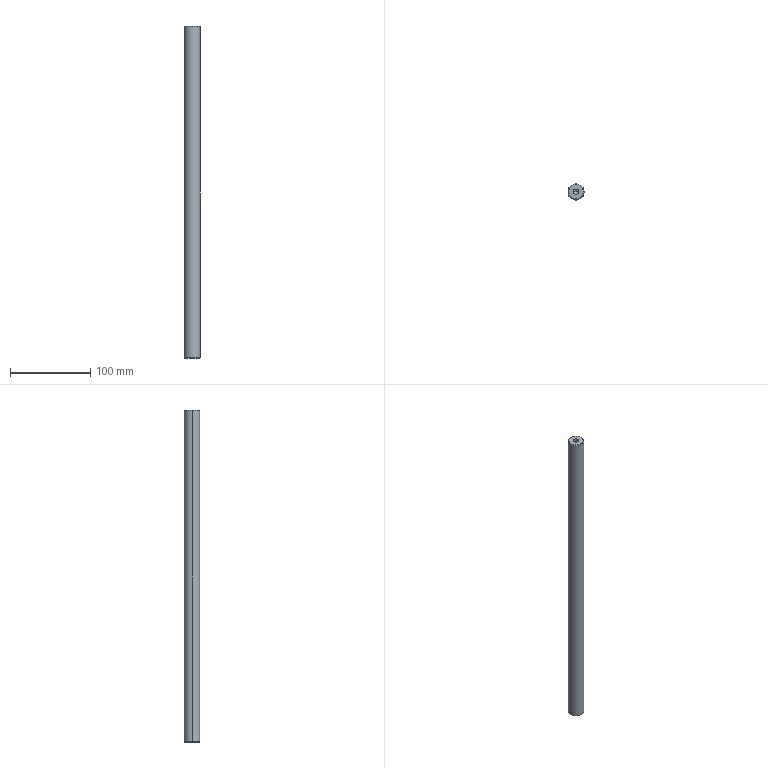Part | SolidWorks | features HoleWzd 2, Chamfer 1, Extrusion 1 | 1 solid | 16 faces | box 20 x 20 x 415 mm | volume 128650 mm3 | cone 8 | cylinder 6 | plane 2 | commonest cylinder face diameters 6.8 x4 20 x2
STEP:
#1=CARTESIAN_POINT('',(3.4,0.,22.25));
#2=VERTEX_POINT('',#1);
#3=CARTESIAN_POINT('',(-3.4,0.,22.25));
#4=VERTEX_POINT('',#3);
#5=CARTESIAN_POINT('',(0.,0.,22.25));
#6=DIRECTION('',(0.,0.,-1.));
#7=DIRECTION('',(-1.,0.,0.));
#8=AXIS2_PLACEMENT_3D('',#5,#6,#7);
#9=CIRCLE('',#8,3.4);
#10=EDGE_CURVE('',#2,#4,#9,.T.);
#11=ORIENTED_EDGE('',*,*,#10,.F.);
#12=CARTESIAN_POINT('',(3.4,0.,0.));
#13=VERTEX_POINT('',#12);
#14=CARTESIAN_POINT('',(3.4,0.,0.));
#15=DIRECTION('',(0.,0.,-1.));
#16=VECTOR('',#15,1000.);
#17=LINE('',#14,#16);
#18=EDGE_CURVE('',#2,#13,#17,.T.);
#19=ORIENTED_EDGE('',*,*,#18,.T.);
#20=CARTESIAN_POINT('',(-3.4,0.,0.));
#21=VERTEX_POINT('',#20);
#22=CARTESIAN_POINT('',(0.,0.,0.));
#23=DIRECTION('',(0.,0.,-1.));
#24=DIRECTION('',(-1.,0.,0.));
#25=AXIS2_PLACEMENT_3D('',#22,#23,#24);
#26=CIRCLE('',#25,3.4);
#27=EDGE_CURVE('',#13,#21,#26,.T.);
#28=ORIENTED_EDGE('',*,*,#27,.T.);
#29=CARTESIAN_POINT('',(-3.4,0.,0.));
#30=DIRECTION('',(0.,0.,-1.));
#31=VECTOR('',#30,1000.);
#32=LINE('',#29,#31);
#33=EDGE_CURVE('',#4,#21,#32,.T.);
#34=ORIENTED_EDGE('',*,*,#33,.F.);
#35=EDGE_LOOP('',(#11,#19,#28,#34));
#36=FACE_OUTER_BOUND('',#35,.T.);
#37=CARTESIAN_POINT('',(0.,0.,0.));
#38=DIRECTION('',(0.,0.,-1.));
#39=DIRECTION('',(-1.,0.,0.));
#40=AXIS2_PLACEMENT_3D('',#37,#38,#39);
#41=CYLINDRICAL_SURFACE('',#40,3.4);
#42=ADVANCED_FACE('',(#36),#41,.F.);
#43=CARTESIAN_POINT('',(0.,0.,24.293));
#44=VERTEX_POINT('',#43);
#45=CARTESIAN_POINT('',(-3.4,0.,22.25));
#46=DIRECTION('',(-0.8572,0.,-0.515));
#47=VECTOR('',#46,1000.);
#48=LINE('',#45,#47);
#49=EDGE_CURVE('',#44,#4,#48,.T.);
#50=ORIENTED_EDGE('',*,*,#49,.F.);
#51=CARTESIAN_POINT('',(3.4,0.,22.25));
#52=DIRECTION('',(0.8572,0.,-0.515));
#53=VECTOR('',#52,1000.);
#54=LINE('',#51,#53);
#55=EDGE_CURVE('',#44,#2,#54,.T.);
#56=ORIENTED_EDGE('',*,*,#55,.T.);
#57=ORIENTED_EDGE('',*,*,#10,.T.);
#58=EDGE_LOOP('',(#50,#56,#57));
#59=FACE_OUTER_BOUND('',#58,.T.);
#60=CARTESIAN_POINT('',(0.,0.,22.25));
#61=DIRECTION('',(0.,0.,-1.));
#62=DIRECTION('',(-1.,0.,0.));
#63=AXIS2_PLACEMENT_3D('',#60,#61,#62);
#64=CONICAL_SURFACE('',#63,3.4,1.03);
#65=ADVANCED_FACE('',(#59),#64,.F.);
#66=CARTESIAN_POINT('',(9.,0.,415.));
#67=VERTEX_POINT('',#66);
#68=CARTESIAN_POINT('',(-9.,0.,415.));
#69=VERTEX_POINT('',#68);
#70=CARTESIAN_POINT('',(0.,0.,415.));
#71=DIRECTION('',(0.,0.,1.));
#72=DIRECTION('',(1.,0.,0.));
#73=AXIS2_PLACEMENT_3D('',#70,#71,#72);
#74=CIRCLE('',#73,9.);
#75=EDGE_CURVE('',#67,#69,#74,.T.);
#76=ORIENTED_EDGE('',*,*,#75,.F.);
#77=CARTESIAN_POINT('',(10.,0.,414.));
#78=VERTEX_POINT('',#77);
#79=CARTESIAN_POINT('',(9.,0.,415.));
#80=DIRECTION('',(0.7071,0.,-0.7071));
#81=VECTOR('',#80,1000.);
#82=LINE('',#79,#81);
#83=EDGE_CURVE('',#67,#78,#82,.T.);
#84=ORIENTED_EDGE('',*,*,#83,.T.);
#85=CARTESIAN_POINT('',(-10.,0.,414.));
#86=VERTEX_POINT('',#85);
#87=CARTESIAN_POINT('',(0.,0.,414.));
#88=DIRECTION('',(0.,0.,-1.));
#89=DIRECTION('',(1.,0.,0.));
#90=AXIS2_PLACEMENT_3D('',#87,#88,#89);
#91=CIRCLE('',#90,10.);
#92=EDGE_CURVE('',#86,#78,#91,.T.);
#93=ORIENTED_EDGE('',*,*,#92,.F.);
#94=CARTESIAN_POINT('',(-9.,0.,415.));
#95=DIRECTION('',(-0.7071,0.,-0.7071));
#96=VECTOR('',#95,1000.);
#97=LINE('',#94,#96);
#98=EDGE_CURVE('',#69,#86,#97,.T.);
#99=ORIENTED_EDGE('',*,*,#98,.F.);
#100=EDGE_LOOP('',(#76,#84,#93,#99));
#101=FACE_OUTER_BOUND('',#100,.T.);
#102=CARTESIAN_POINT('',(0.,0.,415.));
#103=DIRECTION('',(0.,0.,-1.));
#104=DIRECTION('',(-1.,0.,0.));
#105=AXIS2_PLACEMENT_3D('',#102,#103,#104);
#106=CONICAL_SURFACE('',#105,9.,0.7854);
#107=ADVANCED_FACE('',(#101),#106,.T.);
#108=CARTESIAN_POINT('',(-9.,0.,0.));
#109=VERTEX_POINT('',#108);
#110=CARTESIAN_POINT('',(9.,0.,0.));
#111=VERTEX_POINT('',#110);
#112=CARTESIAN_POINT('',(0.,0.,0.));
#113=DIRECTION('',(0.,0.,-1.));
#114=DIRECTION('',(1.,0.,0.));
#115=AXIS2_PLACEMENT_3D('',#112,#113,#114);
#116=CIRCLE('',#115,9.);
#117=EDGE_CURVE('',#109,#111,#116,.T.);
#118=ORIENTED_EDGE('',*,*,#117,.F.);
#119=CARTESIAN_POINT('',(-10.,0.,1.));
#120=VERTEX_POINT('',#119);
#121=CARTESIAN_POINT('',(-10.,0.,1.));
#122=DIRECTION('',(-0.7071,0.,0.7071));
#123=VECTOR('',#122,1000.);
#124=LINE('',#121,#123);
#125=EDGE_CURVE('',#109,#120,#124,.T.);
#126=ORIENTED_EDGE('',*,*,#125,.T.);
#127=CARTESIAN_POINT('',(10.,0.,1.));
#128=VERTEX_POINT('',#127);
#129=CARTESIAN_POINT('',(0.,0.,1.));
#130=DIRECTION('',(0.,0.,1.));
#131=DIRECTION('',(1.,0.,0.));
#132=AXIS2_PLACEMENT_3D('',#129,#130,#131);
#133=CIRCLE('',#132,10.);
#134=EDGE_CURVE('',#128,#120,#133,.T.);
#135=ORIENTED_EDGE('',*,*,#134,.F.);
#136=CARTESIAN_POINT('',(10.,0.,1.));
#137=DIRECTION('',(0.7071,0.,0.7071));
#138=VECTOR('',#137,1000.);
#139=LINE('',#136,#138);
#140=EDGE_CURVE('',#111,#128,#139,.T.);
#141=ORIENTED_EDGE('',*,*,#140,.F.);
#142=EDGE_LOOP('',(#118,#126,#135,#141));
#143=FACE_OUTER_BOUND('',#142,.T.);
#144=CARTESIAN_POINT('',(0.,0.,1.));
#145=DIRECTION('',(0.,0.,1.));
#146=DIRECTION('',(1.,0.,0.));
#147=AXIS2_PLACEMENT_3D('',#144,#145,#146);
#148=CONICAL_SURFACE('',#147,10.,0.7854);
#149=ADVANCED_FACE('',(#143),#148,.T.);
#150=CARTESIAN_POINT('',(-3.4,0.,392.75));
#151=VERTEX_POINT('',#150);
#152=CARTESIAN_POINT('',(3.4,0.,392.75));
#153=VERTEX_POINT('',#152);
#154=CARTESIAN_POINT('',(0.,0.,392.75));
#155=DIRECTION('',(0.,0.,1.));
#156=DIRECTION('',(1.,0.,0.));
#157=AXIS2_PLACEMENT_3D('',#154,#155,#156);
#158=CIRCLE('',#157,3.4);
#159=EDGE_CURVE('',#151,#153,#158,.T.);
#160=ORIENTED_EDGE('',*,*,#159,.F.);
#161=CARTESIAN_POINT('',(-3.4,0.,415.));
#162=VERTEX_POINT('',#161);
#163=CARTESIAN_POINT('',(-3.4,0.,415.));
#164=DIRECTION('',(0.,0.,1.));
#165=VECTOR('',#164,1000.);
#166=LINE('',#163,#165);
#167=EDGE_CURVE('',#151,#162,#166,.T.);
#168=ORIENTED_EDGE('',*,*,#167,.T.);
#169=CARTESIAN_POINT('',(3.4,0.,415.));
#170=VERTEX_POINT('',#169);
#171=CARTESIAN_POINT('',(0.,0.,415.));
#172=DIRECTION('',(0.,0.,1.));
#173=DIRECTION('',(1.,0.,0.));
#174=AXIS2_PLACEMENT_3D('',#171,#172,#173);
#175=CIRCLE('',#174,3.4);
#176=EDGE_CURVE('',#162,#170,#175,.T.);
#177=ORIENTED_EDGE('',*,*,#176,.T.);
#178=CARTESIAN_POINT('',(3.4,0.,415.));
#179=DIRECTION('',(0.,0.,1.));
#180=VECTOR('',#179,1000.);
#181=LINE('',#178,#180);
#182=EDGE_CURVE('',#153,#170,#181,.T.);
#183=ORIENTED_EDGE('',*,*,#182,.F.);
#184=EDGE_LOOP('',(#160,#168,#177,#183));
#185=FACE_OUTER_BOUND('',#184,.T.);
#186=CARTESIAN_POINT('',(0.,0.,415.));
#187=DIRECTION('',(0.,0.,1.));
#188=DIRECTION('',(1.,0.,0.));
#189=AXIS2_PLACEMENT_3D('',#186,#187,#188);
#190=CYLINDRICAL_SURFACE('',#189,3.4);
#191=ADVANCED_FACE('',(#185),#190,.F.);
#192=CARTESIAN_POINT('',(0.,0.,390.707));
#193=VERTEX_POINT('',#192);
#194=CARTESIAN_POINT('',(3.4,0.,392.75));
#195=DIRECTION('',(0.8572,0.,0.515));
#196=VECTOR('',#195,1000.);
#197=LINE('',#194,#196);
#198=EDGE_CURVE('',#193,#153,#197,.T.);
#199=ORIENTED_EDGE('',*,*,#198,.F.);
#200=CARTESIAN_POINT('',(-3.4,0.,392.75));
#201=DIRECTION('',(-0.8572,0.,0.515));
#202=VECTOR('',#201,1000.);
#203=LINE('',#200,#202);
#204=EDGE_CURVE('',#193,#151,#203,.T.);
#205=ORIENTED_EDGE('',*,*,#204,.T.);
#206=ORIENTED_EDGE('',*,*,#159,.T.);
#207=EDGE_LOOP('',(#199,#205,#206));
#208=FACE_OUTER_BOUND('',#207,.T.);
#209=CARTESIAN_POINT('',(0.,0.,392.75));
#210=DIRECTION('',(0.,0.,1.));
#211=DIRECTION('',(1.,0.,0.));
#212=AXIS2_PLACEMENT_3D('',#209,#210,#211);
#213=CONICAL_SURFACE('',#212,3.4,1.03);
#214=ADVANCED_FACE('',(#208),#213,.F.);
#215=ORIENTED_EDGE('',*,*,#92,.T.);
#216=CARTESIAN_POINT('',(10.,0.,415.));
#217=DIRECTION('',(0.,0.,-1.));
#218=VECTOR('',#217,1000.);
#219=LINE('',#216,#218);
#220=EDGE_CURVE('',#78,#128,#219,.T.);
#221=ORIENTED_EDGE('',*,*,#220,.T.);
#222=ORIENTED_EDGE('',*,*,#134,.T.);
#223=CARTESIAN_POINT('',(-10.,0.,415.));
#224=DIRECTION('',(0.,0.,-1.));
#225=VECTOR('',#224,1000.);
#226=LINE('',#223,#225);
#227=EDGE_CURVE('',#86,#120,#226,.T.);
#228=ORIENTED_EDGE('',*,*,#227,.F.);
#229=EDGE_LOOP('',(#215,#221,#222,#228));
#230=FACE_OUTER_BOUND('',#229,.T.);
#231=CARTESIAN_POINT('',(0.,0.,415.));
#232=DIRECTION('',(0.,0.,-1.));
#233=DIRECTION('',(-1.,0.,0.));
#234=AXIS2_PLACEMENT_3D('',#231,#232,#233);
#235=CYLINDRICAL_SURFACE('',#234,10.);
#236=ADVANCED_FACE('',(#230),#235,.T.);
#237=ORIENTED_EDGE('',*,*,#220,.F.);
#238=CARTESIAN_POINT('',(0.,0.,414.));
#239=DIRECTION('',(0.,0.,-1.));
#240=DIRECTION('',(1.,0.,0.));
#241=AXIS2_PLACEMENT_3D('',#238,#239,#240);
#242=CIRCLE('',#241,10.);
#243=EDGE_CURVE('',#78,#86,#242,.T.);
#244=ORIENTED_EDGE('',*,*,#243,.T.);
#245=ORIENTED_EDGE('',*,*,#227,.T.);
#246=CARTESIAN_POINT('',(0.,0.,1.));
#247=DIRECTION('',(0.,0.,1.));
#248=DIRECTION('',(1.,0.,0.));
#249=AXIS2_PLACEMENT_3D('',#246,#247,#248);
#250=CIRCLE('',#249,10.);
#251=EDGE_CURVE('',#120,#128,#250,.T.);
#252=ORIENTED_EDGE('',*,*,#251,.T.);
#253=EDGE_LOOP('',(#237,#244,#245,#252));
#254=FACE_OUTER_BOUND('',#253,.T.);
#255=CARTESIAN_POINT('',(0.,0.,415.));
#256=DIRECTION('',(0.,0.,-1.));
#257=DIRECTION('',(-1.,0.,0.));
#258=AXIS2_PLACEMENT_3D('',#255,#256,#257);
#259=CYLINDRICAL_SURFACE('',#258,10.);
#260=ADVANCED_FACE('',(#254),#259,.T.);
#261=CARTESIAN_POINT('',(0.,0.,415.));
#262=DIRECTION('',(0.,0.,1.));
#263=DIRECTION('',(1.,0.,0.));
#264=AXIS2_PLACEMENT_3D('',#261,#262,#263);
#265=CIRCLE('',#264,9.);
#266=EDGE_CURVE('',#69,#67,#265,.T.);
#267=ORIENTED_EDGE('',*,*,#266,.T.);
#268=ORIENTED_EDGE('',*,*,#75,.T.);
#269=EDGE_LOOP('',(#267,#268));
#270=FACE_OUTER_BOUND('',#269,.T.);
#271=CARTESIAN_POINT('',(0.,0.,415.));
#272=DIRECTION('',(0.,0.,1.));
#273=DIRECTION('',(1.,0.,0.));
#274=AXIS2_PLACEMENT_3D('',#271,#272,#273);
#275=CIRCLE('',#274,3.4);
#276=EDGE_CURVE('',#170,#162,#275,.T.);
#277=ORIENTED_EDGE('',*,*,#276,.F.);
#278=ORIENTED_EDGE('',*,*,#176,.F.);
#279=EDGE_LOOP('',(#277,#278));
#280=FACE_BOUND('',#279,.T.);
#281=CARTESIAN_POINT('',(0.,0.,415.));
#282=DIRECTION('',(0.,0.,1.));
#283=DIRECTION('',(1.,0.,0.));
#284=AXIS2_PLACEMENT_3D('',#281,#282,#283);
#285=PLANE('',#284);
#286=ADVANCED_FACE('',(#270,#280),#285,.T.);
#287=CARTESIAN_POINT('',(0.,0.,0.));
#288=DIRECTION('',(0.,0.,-1.));
#289=DIRECTION('',(-1.,0.,0.));
#290=AXIS2_PLACEMENT_3D('',#287,#288,#289);
#291=CIRCLE('',#290,3.4);
#292=EDGE_CURVE('',#21,#13,#291,.T.);
#293=ORIENTED_EDGE('',*,*,#292,.F.);
#294=ORIENTED_EDGE('',*,*,#27,.F.);
#295=EDGE_LOOP('',(#293,#294));
#296=FACE_BOUND('',#295,.T.);
#297=CARTESIAN_POINT('',(0.,0.,0.));
#298=DIRECTION('',(0.,0.,-1.));
#299=DIRECTION('',(1.,0.,0.));
#300=AXIS2_PLACEMENT_3D('',#297,#298,#299);
#301=CIRCLE('',#300,9.);
#302=EDGE_CURVE('',#111,#109,#301,.T.);
#303=ORIENTED_EDGE('',*,*,#302,.T.);
#304=ORIENTED_EDGE('',*,*,#117,.T.);
#305=EDGE_LOOP('',(#303,#304));
#306=FACE_OUTER_BOUND('',#305,.T.);
#307=CARTESIAN_POINT('',(0.,0.,0.));
#308=DIRECTION('',(0.,0.,1.));
#309=DIRECTION('',(1.,0.,0.));
#310=AXIS2_PLACEMENT_3D('',#307,#308,#309);
#311=PLANE('',#310);
#312=ADVANCED_FACE('',(#296,#306),#311,.F.);
#313=ORIENTED_EDGE('',*,*,#204,.F.);
#314=ORIENTED_EDGE('',*,*,#198,.T.);
#315=CARTESIAN_POINT('',(0.,0.,392.75));
#316=DIRECTION('',(0.,0.,1.));
#317=DIRECTION('',(1.,0.,0.));
#318=AXIS2_PLACEMENT_3D('',#315,#316,#317);
#319=CIRCLE('',#318,3.4);
#320=EDGE_CURVE('',#153,#151,#319,.T.);
#321=ORIENTED_EDGE('',*,*,#320,.T.);
#322=EDGE_LOOP('',(#313,#314,#321));
#323=FACE_OUTER_BOUND('',#322,.T.);
#324=CARTESIAN_POINT('',(0.,0.,392.75));
#325=DIRECTION('',(0.,0.,1.));
#326=DIRECTION('',(1.,0.,0.));
#327=AXIS2_PLACEMENT_3D('',#324,#325,#326);
#328=CONICAL_SURFACE('',#327,3.4,1.03);
#329=ADVANCED_FACE('',(#323),#328,.F.);
#330=ORIENTED_EDGE('',*,*,#167,.F.);
#331=ORIENTED_EDGE('',*,*,#320,.F.);
#332=ORIENTED_EDGE('',*,*,#182,.T.);
#333=ORIENTED_EDGE('',*,*,#276,.T.);
#334=EDGE_LOOP('',(#330,#331,#332,#333));
#335=FACE_OUTER_BOUND('',#334,.T.);
#336=CARTESIAN_POINT('',(0.,0.,415.));
#337=DIRECTION('',(0.,0.,1.));
#338=DIRECTION('',(1.,0.,0.));
#339=AXIS2_PLACEMENT_3D('',#336,#337,#338);
#340=CYLINDRICAL_SURFACE('',#339,3.4);
#341=ADVANCED_FACE('',(#335),#340,.F.);
#342=ORIENTED_EDGE('',*,*,#125,.F.);
#343=ORIENTED_EDGE('',*,*,#302,.F.);
#344=ORIENTED_EDGE('',*,*,#140,.T.);
#345=ORIENTED_EDGE('',*,*,#251,.F.);
#346=EDGE_LOOP('',(#342,#343,#344,#345));
#347=FACE_OUTER_BOUND('',#346,.T.);
#348=CARTESIAN_POINT('',(0.,0.,1.));
#349=DIRECTION('',(0.,0.,1.));
#350=DIRECTION('',(1.,0.,0.));
#351=AXIS2_PLACEMENT_3D('',#348,#349,#350);
#352=CONICAL_SURFACE('',#351,10.,0.7854);
#353=ADVANCED_FACE('',(#347),#352,.T.);
#354=ORIENTED_EDGE('',*,*,#83,.F.);
#355=ORIENTED_EDGE('',*,*,#266,.F.);
#356=ORIENTED_EDGE('',*,*,#98,.T.);
#357=ORIENTED_EDGE('',*,*,#243,.F.);
#358=EDGE_LOOP('',(#354,#355,#356,#357));
#359=FACE_OUTER_BOUND('',#358,.T.);
#360=CARTESIAN_POINT('',(0.,0.,415.));
#361=DIRECTION('',(0.,0.,-1.));
#362=DIRECTION('',(-1.,0.,0.));
#363=AXIS2_PLACEMENT_3D('',#360,#361,#362);
#364=CONICAL_SURFACE('',#363,9.,0.7854);
#365=ADVANCED_FACE('',(#359),#364,.T.);
#366=ORIENTED_EDGE('',*,*,#55,.F.);
#367=ORIENTED_EDGE('',*,*,#49,.T.);
#368=CARTESIAN_POINT('',(0.,0.,22.25));
#369=DIRECTION('',(0.,0.,-1.));
#370=DIRECTION('',(-1.,0.,0.));
#371=AXIS2_PLACEMENT_3D('',#368,#369,#370);
#372=CIRCLE('',#371,3.4);
#373=EDGE_CURVE('',#4,#2,#372,.T.);
#374=ORIENTED_EDGE('',*,*,#373,.T.);
#375=EDGE_LOOP('',(#366,#367,#374));
#376=FACE_OUTER_BOUND('',#375,.T.);
#377=CARTESIAN_POINT('',(0.,0.,22.25));
#378=DIRECTION('',(0.,0.,-1.));
#379=DIRECTION('',(-1.,0.,0.));
#380=AXIS2_PLACEMENT_3D('',#377,#378,#379);
#381=CONICAL_SURFACE('',#380,3.4,1.03);
#382=ADVANCED_FACE('',(#376),#381,.F.);
#383=ORIENTED_EDGE('',*,*,#18,.F.);
#384=ORIENTED_EDGE('',*,*,#373,.F.);
#385=ORIENTED_EDGE('',*,*,#33,.T.);
#386=ORIENTED_EDGE('',*,*,#292,.T.);
#387=EDGE_LOOP('',(#383,#384,#385,#386));
#388=FACE_OUTER_BOUND('',#387,.T.);
#389=CARTESIAN_POINT('',(0.,0.,0.));
#390=DIRECTION('',(0.,0.,-1.));
#391=DIRECTION('',(-1.,0.,0.));
#392=AXIS2_PLACEMENT_3D('',#389,#390,#391);
#393=CYLINDRICAL_SURFACE('',#392,3.4);
#394=ADVANCED_FACE('',(#388),#393,.F.);
#395=CLOSED_SHELL('',(#42,#65,#107,#149,#191,#214,#236,#260,#286,#312,#329,#341,#353,#365,#382,#394));
#396=MANIFOLD_SOLID_BREP('',#395);
#397=CARTESIAN_POINT('',(0.,0.,0.));
#398=DIRECTION('',(0.,0.,1.));
#399=DIRECTION('',(1.,0.,0.));
#400=AXIS2_PLACEMENT_3D('',#397,#398,#399);
#401=(LENGTH_UNIT()NAMED_UNIT(*)SI_UNIT(.MILLI.,.METRE.));
#402=UNCERTAINTY_MEASURE_WITH_UNIT(LENGTH_MEASURE(0.00001),#401,'','');
#403=(NAMED_UNIT(*)PLANE_ANGLE_UNIT()SI_UNIT($,.RADIAN.));
#404=(NAMED_UNIT(*)SI_UNIT($,.STERADIAN.)SOLID_ANGLE_UNIT());
#405=(GEOMETRIC_REPRESENTATION_CONTEXT(3)GLOBAL_UNCERTAINTY_ASSIGNED_CONTEXT((#402))GLOBAL_UNIT_ASSIGNED_CONTEXT((#401,#403,#404))REPRESENTATION_CONTEXT('',''));
#406=ADVANCED_BREP_SHAPE_REPRESENTATION('',(#396,#400),#405);